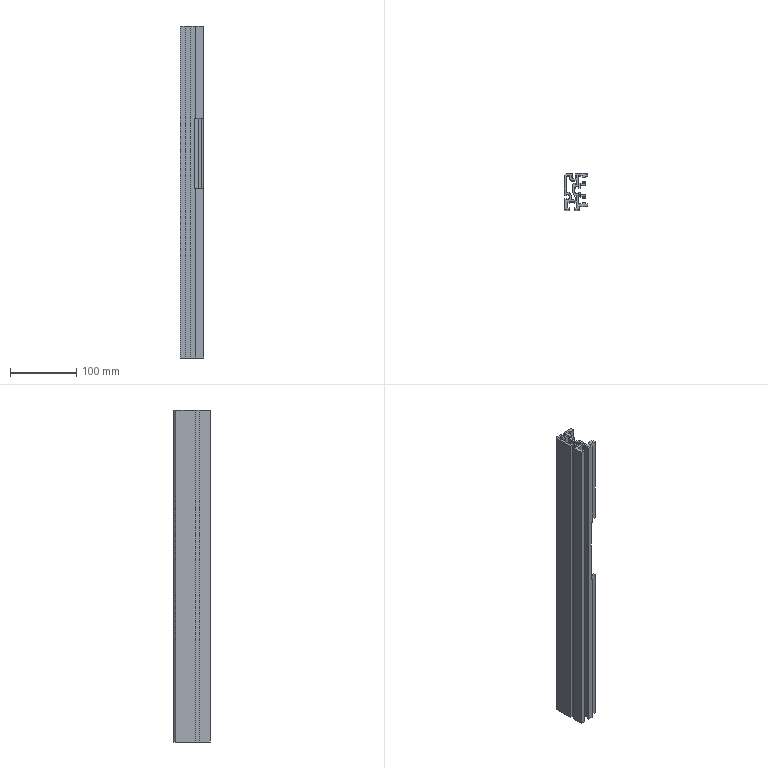Part | STEP file | 1 solid | 174 faces | box 35 x 55 x 500 mm | volume 378713 mm3 | plane 128 | cylinder 37 | cone 9 | commonest cylinder face diameters 2.5 x9 2 x8 6.5 x6 2.3 x4 11 x4 24 x4